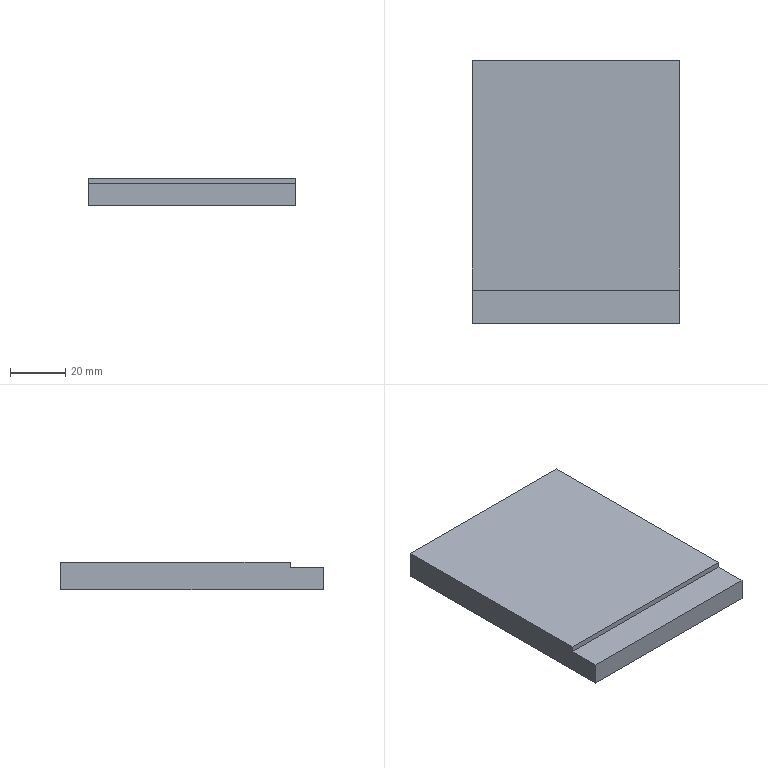Part | STEP file | 001-004-Feeding mechanism fixing plate | 1 solid | 8 faces | box 75 x 95 x 10 mm | volume 69450 mm3 | plane 8
STEP:
#1=CARTESIAN_POINT('',(0.,0.,0.));
#2=DIRECTION('',(0.,0.,1.));
#3=DIRECTION('',(1.,0.,0.));
#4=AXIS2_PLACEMENT_3D('',#1,#2,#3);
#5=CARTESIAN_POINT('',(37.5,-35.5,10.));
#6=VERTEX_POINT('',#5);
#7=CARTESIAN_POINT('',(37.5,47.5,10.));
#8=VERTEX_POINT('',#7);
#9=CARTESIAN_POINT('',(37.5,-47.5,10.));
#10=DIRECTION('',(0.,1.,0.));
#11=VECTOR('',#10,1.);
#12=LINE('',#9,#11);
#13=CARTESIAN_POINT('',(37.5,-47.5,10.));
#14=DIRECTION('',(-1.,0.,0.));
#15=DIRECTION('',(0.,0.,1.));
#16=AXIS2_PLACEMENT_3D('',#13,#14,#15);
#17=PLANE('',#16);
#18=CARTESIAN_POINT('',(0.,0.));
#19=DIRECTION('',(0.,1.));
#20=VECTOR('',#19,1.);
#21=LINE('',#18,#20);
#22=(GEOMETRIC_REPRESENTATION_CONTEXT(2)PARAMETRIC_REPRESENTATION_CONTEXT()REPRESENTATION_CONTEXT('',''));
#23=DEFINITIONAL_REPRESENTATION('',(#21),#22);
#24=PCURVE('',#17,#23);
#25=CARTESIAN_POINT('',(0.,0.,10.));
#26=DIRECTION('',(0.,0.,-1.));
#27=DIRECTION('',(-1.,0.,0.));
#28=AXIS2_PLACEMENT_3D('',#25,#26,#27);
#29=PLANE('',#28);
#30=CARTESIAN_POINT('',(-37.5,-47.5));
#31=DIRECTION('',(0.,1.));
#32=VECTOR('',#31,1.);
#33=LINE('',#30,#32);
#34=(GEOMETRIC_REPRESENTATION_CONTEXT(2)PARAMETRIC_REPRESENTATION_CONTEXT()REPRESENTATION_CONTEXT('',''));
#35=DEFINITIONAL_REPRESENTATION('',(#33),#34);
#36=PCURVE('',#29,#35);
#37=SURFACE_CURVE('',#12,(#24,#36),.PCURVE_S1.);
#38=EDGE_CURVE('',#6,#8,#37,.T.);
#39=ORIENTED_EDGE('',*,*,#38,.F.);
#40=CARTESIAN_POINT('',(37.5,-35.5,8.));
#41=VERTEX_POINT('',#40);
#42=CARTESIAN_POINT('',(37.5,-35.5,8.));
#43=DIRECTION('',(0.,0.,1.));
#44=VECTOR('',#43,1.);
#45=LINE('',#42,#44);
#46=CARTESIAN_POINT('',(-2.,12.));
#47=DIRECTION('',(1.,0.));
#48=VECTOR('',#47,1.);
#49=LINE('',#46,#48);
#50=(GEOMETRIC_REPRESENTATION_CONTEXT(2)PARAMETRIC_REPRESENTATION_CONTEXT()REPRESENTATION_CONTEXT('',''));
#51=DEFINITIONAL_REPRESENTATION('',(#49),#50);
#52=PCURVE('',#17,#51);
#53=CARTESIAN_POINT('',(-37.5,-35.5,8.));
#54=DIRECTION('',(0.,1.,0.));
#55=DIRECTION('',(0.,0.,1.));
#56=AXIS2_PLACEMENT_3D('',#53,#54,#55);
#57=PLANE('',#56);
#58=CARTESIAN_POINT('',(0.,75.));
#59=DIRECTION('',(1.,0.));
#60=VECTOR('',#59,1.);
#61=LINE('',#58,#60);
#62=(GEOMETRIC_REPRESENTATION_CONTEXT(2)PARAMETRIC_REPRESENTATION_CONTEXT()REPRESENTATION_CONTEXT('',''));
#63=DEFINITIONAL_REPRESENTATION('',(#61),#62);
#64=PCURVE('',#57,#63);
#65=SURFACE_CURVE('',#45,(#52,#64),.PCURVE_S1.);
#66=EDGE_CURVE('',#41,#6,#65,.T.);
#67=ORIENTED_EDGE('',*,*,#66,.F.);
#68=CARTESIAN_POINT('',(37.5,-47.5,8.));
#69=VERTEX_POINT('',#68);
#70=CARTESIAN_POINT('',(37.5,-47.5,8.));
#71=DIRECTION('',(0.,1.,0.));
#72=VECTOR('',#71,1.);
#73=LINE('',#70,#72);
#74=CARTESIAN_POINT('',(-2.,0.));
#75=DIRECTION('',(0.,1.));
#76=VECTOR('',#75,1.);
#77=LINE('',#74,#76);
#78=(GEOMETRIC_REPRESENTATION_CONTEXT(2)PARAMETRIC_REPRESENTATION_CONTEXT()REPRESENTATION_CONTEXT('',''));
#79=DEFINITIONAL_REPRESENTATION('',(#77),#78);
#80=PCURVE('',#17,#79);
#81=CARTESIAN_POINT('',(0.,0.,8.));
#82=DIRECTION('',(0.,0.,-1.));
#83=DIRECTION('',(-1.,0.,0.));
#84=AXIS2_PLACEMENT_3D('',#81,#82,#83);
#85=PLANE('',#84);
#86=CARTESIAN_POINT('',(-37.5,-47.5));
#87=DIRECTION('',(0.,1.));
#88=VECTOR('',#87,1.);
#89=LINE('',#86,#88);
#90=(GEOMETRIC_REPRESENTATION_CONTEXT(2)PARAMETRIC_REPRESENTATION_CONTEXT()REPRESENTATION_CONTEXT('',''));
#91=DEFINITIONAL_REPRESENTATION('',(#89),#90);
#92=PCURVE('',#85,#91);
#93=SURFACE_CURVE('',#73,(#80,#92),.PCURVE_S1.);
#94=EDGE_CURVE('',#69,#41,#93,.T.);
#95=ORIENTED_EDGE('',*,*,#94,.F.);
#96=CARTESIAN_POINT('',(37.5,-47.5,0.));
#97=VERTEX_POINT('',#96);
#98=CARTESIAN_POINT('',(37.5,-47.5,10.));
#99=DIRECTION('',(0.,0.,-1.));
#100=VECTOR('',#99,1.);
#101=LINE('',#98,#100);
#102=CARTESIAN_POINT('',(0.,0.));
#103=DIRECTION('',(-1.,0.));
#104=VECTOR('',#103,1.);
#105=LINE('',#102,#104);
#106=(GEOMETRIC_REPRESENTATION_CONTEXT(2)PARAMETRIC_REPRESENTATION_CONTEXT()REPRESENTATION_CONTEXT('',''));
#107=DEFINITIONAL_REPRESENTATION('',(#105),#106);
#108=PCURVE('',#17,#107);
#109=CARTESIAN_POINT('',(-37.5,-47.5,10.));
#110=DIRECTION('',(0.,1.,0.));
#111=DIRECTION('',(0.,0.,1.));
#112=AXIS2_PLACEMENT_3D('',#109,#110,#111);
#113=PLANE('',#112);
#114=CARTESIAN_POINT('',(0.,75.));
#115=DIRECTION('',(-1.,0.));
#116=VECTOR('',#115,1.);
#117=LINE('',#114,#116);
#118=(GEOMETRIC_REPRESENTATION_CONTEXT(2)PARAMETRIC_REPRESENTATION_CONTEXT()REPRESENTATION_CONTEXT('',''));
#119=DEFINITIONAL_REPRESENTATION('',(#117),#118);
#120=PCURVE('',#113,#119);
#121=SURFACE_CURVE('',#101,(#108,#120),.PCURVE_S1.);
#122=EDGE_CURVE('',#69,#97,#121,.T.);
#123=ORIENTED_EDGE('',*,*,#122,.T.);
#124=CARTESIAN_POINT('',(37.5,47.5,0.));
#125=VERTEX_POINT('',#124);
#126=CARTESIAN_POINT('',(37.5,-47.5,0.));
#127=DIRECTION('',(0.,1.,0.));
#128=VECTOR('',#127,1.);
#129=LINE('',#126,#128);
#130=CARTESIAN_POINT('',(-10.,0.));
#131=DIRECTION('',(0.,1.));
#132=VECTOR('',#131,1.);
#133=LINE('',#130,#132);
#134=(GEOMETRIC_REPRESENTATION_CONTEXT(2)PARAMETRIC_REPRESENTATION_CONTEXT()REPRESENTATION_CONTEXT('',''));
#135=DEFINITIONAL_REPRESENTATION('',(#133),#134);
#136=PCURVE('',#17,#135);
#137=CARTESIAN_POINT('',(0.,0.,0.));
#138=DIRECTION('',(0.,0.,-1.));
#139=DIRECTION('',(-1.,0.,0.));
#140=AXIS2_PLACEMENT_3D('',#137,#138,#139);
#141=PLANE('',#140);
#142=CARTESIAN_POINT('',(-37.5,-47.5));
#143=DIRECTION('',(0.,1.));
#144=VECTOR('',#143,1.);
#145=LINE('',#142,#144);
#146=(GEOMETRIC_REPRESENTATION_CONTEXT(2)PARAMETRIC_REPRESENTATION_CONTEXT()REPRESENTATION_CONTEXT('',''));
#147=DEFINITIONAL_REPRESENTATION('',(#145),#146);
#148=PCURVE('',#141,#147);
#149=SURFACE_CURVE('',#129,(#136,#148),.PCURVE_S1.);
#150=EDGE_CURVE('',#97,#125,#149,.T.);
#151=ORIENTED_EDGE('',*,*,#150,.T.);
#152=CARTESIAN_POINT('',(37.5,47.5,10.));
#153=DIRECTION('',(0.,0.,-1.));
#154=VECTOR('',#153,1.);
#155=LINE('',#152,#154);
#156=CARTESIAN_POINT('',(0.,95.));
#157=DIRECTION('',(-1.,0.));
#158=VECTOR('',#157,1.);
#159=LINE('',#156,#158);
#160=(GEOMETRIC_REPRESENTATION_CONTEXT(2)PARAMETRIC_REPRESENTATION_CONTEXT()REPRESENTATION_CONTEXT('',''));
#161=DEFINITIONAL_REPRESENTATION('',(#159),#160);
#162=PCURVE('',#17,#161);
#163=CARTESIAN_POINT('',(-37.5,47.5,10.));
#164=DIRECTION('',(0.,-1.,0.));
#165=DIRECTION('',(0.,0.,-1.));
#166=AXIS2_PLACEMENT_3D('',#163,#164,#165);
#167=PLANE('',#166);
#168=CARTESIAN_POINT('',(0.,75.));
#169=DIRECTION('',(1.,0.));
#170=VECTOR('',#169,1.);
#171=LINE('',#168,#170);
#172=(GEOMETRIC_REPRESENTATION_CONTEXT(2)PARAMETRIC_REPRESENTATION_CONTEXT()REPRESENTATION_CONTEXT('',''));
#173=DEFINITIONAL_REPRESENTATION('',(#171),#172);
#174=PCURVE('',#167,#173);
#175=SURFACE_CURVE('',#155,(#162,#174),.PCURVE_S1.);
#176=EDGE_CURVE('',#8,#125,#175,.T.);
#177=ORIENTED_EDGE('',*,*,#176,.F.);
#178=EDGE_LOOP('',(#39,#67,#95,#123,#151,#177));
#179=FACE_BOUND('',#178,.T.);
#180=ADVANCED_FACE('',(#179),#17,.F.);
#181=CARTESIAN_POINT('',(-37.5,47.5,0.));
#182=VERTEX_POINT('',#181);
#183=CARTESIAN_POINT('',(-37.5,47.5,0.));
#184=DIRECTION('',(-1.,0.,0.));
#185=VECTOR('',#184,1.);
#186=LINE('',#183,#185);
#187=CARTESIAN_POINT('',(10.,0.));
#188=DIRECTION('',(0.,-1.));
#189=VECTOR('',#188,1.);
#190=LINE('',#187,#189);
#191=(GEOMETRIC_REPRESENTATION_CONTEXT(2)PARAMETRIC_REPRESENTATION_CONTEXT()REPRESENTATION_CONTEXT('',''));
#192=DEFINITIONAL_REPRESENTATION('',(#190),#191);
#193=PCURVE('',#167,#192);
#194=CARTESIAN_POINT('',(37.5,47.5));
#195=DIRECTION('',(1.,0.));
#196=VECTOR('',#195,1.);
#197=LINE('',#194,#196);
#198=(GEOMETRIC_REPRESENTATION_CONTEXT(2)PARAMETRIC_REPRESENTATION_CONTEXT()REPRESENTATION_CONTEXT('',''));
#199=DEFINITIONAL_REPRESENTATION('',(#197),#198);
#200=PCURVE('',#141,#199);
#201=SURFACE_CURVE('',#186,(#193,#200),.PCURVE_S1.);
#202=EDGE_CURVE('',#125,#182,#201,.T.);
#203=ORIENTED_EDGE('',*,*,#202,.T.);
#204=CARTESIAN_POINT('',(-37.5,47.5,10.));
#205=VERTEX_POINT('',#204);
#206=CARTESIAN_POINT('',(-37.5,47.5,10.));
#207=DIRECTION('',(0.,0.,-1.));
#208=VECTOR('',#207,1.);
#209=LINE('',#206,#208);
#210=CARTESIAN_POINT('',(0.,0.));
#211=DIRECTION('',(1.,0.));
#212=VECTOR('',#211,1.);
#213=LINE('',#210,#212);
#214=(GEOMETRIC_REPRESENTATION_CONTEXT(2)PARAMETRIC_REPRESENTATION_CONTEXT()REPRESENTATION_CONTEXT('',''));
#215=DEFINITIONAL_REPRESENTATION('',(#213),#214);
#216=PCURVE('',#167,#215);
#217=CARTESIAN_POINT('',(-37.5,-47.5,10.));
#218=DIRECTION('',(1.,0.,0.));
#219=DIRECTION('',(0.,0.,-1.));
#220=AXIS2_PLACEMENT_3D('',#217,#218,#219);
#221=PLANE('',#220);
#222=CARTESIAN_POINT('',(0.,95.));
#223=DIRECTION('',(1.,0.));
#224=VECTOR('',#223,1.);
#225=LINE('',#222,#224);
#226=(GEOMETRIC_REPRESENTATION_CONTEXT(2)PARAMETRIC_REPRESENTATION_CONTEXT()REPRESENTATION_CONTEXT('',''));
#227=DEFINITIONAL_REPRESENTATION('',(#225),#226);
#228=PCURVE('',#221,#227);
#229=SURFACE_CURVE('',#209,(#216,#228),.PCURVE_S1.);
#230=EDGE_CURVE('',#205,#182,#229,.T.);
#231=ORIENTED_EDGE('',*,*,#230,.F.);
#232=CARTESIAN_POINT('',(-37.5,47.5,10.));
#233=DIRECTION('',(-1.,0.,0.));
#234=VECTOR('',#233,1.);
#235=LINE('',#232,#234);
#236=CARTESIAN_POINT('',(0.,0.));
#237=DIRECTION('',(0.,-1.));
#238=VECTOR('',#237,1.);
#239=LINE('',#236,#238);
#240=(GEOMETRIC_REPRESENTATION_CONTEXT(2)PARAMETRIC_REPRESENTATION_CONTEXT()REPRESENTATION_CONTEXT('',''));
#241=DEFINITIONAL_REPRESENTATION('',(#239),#240);
#242=PCURVE('',#167,#241);
#243=CARTESIAN_POINT('',(37.5,47.5));
#244=DIRECTION('',(1.,0.));
#245=VECTOR('',#244,1.);
#246=LINE('',#243,#245);
#247=(GEOMETRIC_REPRESENTATION_CONTEXT(2)PARAMETRIC_REPRESENTATION_CONTEXT()REPRESENTATION_CONTEXT('',''));
#248=DEFINITIONAL_REPRESENTATION('',(#246),#247);
#249=PCURVE('',#29,#248);
#250=SURFACE_CURVE('',#235,(#242,#249),.PCURVE_S1.);
#251=EDGE_CURVE('',#8,#205,#250,.T.);
#252=ORIENTED_EDGE('',*,*,#251,.F.);
#253=ORIENTED_EDGE('',*,*,#176,.T.);
#254=EDGE_LOOP('',(#203,#231,#252,#253));
#255=FACE_BOUND('',#254,.T.);
#256=ADVANCED_FACE('',(#255),#167,.F.);
#257=CARTESIAN_POINT('',(-37.5,-35.5,8.));
#258=VERTEX_POINT('',#257);
#259=CARTESIAN_POINT('',(-37.5,-47.5,8.));
#260=VERTEX_POINT('',#259);
#261=CARTESIAN_POINT('',(-37.5,-47.5,8.));
#262=DIRECTION('',(0.,-1.,0.));
#263=VECTOR('',#262,1.);
#264=LINE('',#261,#263);
#265=CARTESIAN_POINT('',(2.,0.));
#266=DIRECTION('',(0.,-1.));
#267=VECTOR('',#266,1.);
#268=LINE('',#265,#267);
#269=(GEOMETRIC_REPRESENTATION_CONTEXT(2)PARAMETRIC_REPRESENTATION_CONTEXT()REPRESENTATION_CONTEXT('',''));
#270=DEFINITIONAL_REPRESENTATION('',(#268),#269);
#271=PCURVE('',#221,#270);
#272=CARTESIAN_POINT('',(37.5,-47.5));
#273=DIRECTION('',(0.,-1.));
#274=VECTOR('',#273,1.);
#275=LINE('',#272,#274);
#276=(GEOMETRIC_REPRESENTATION_CONTEXT(2)PARAMETRIC_REPRESENTATION_CONTEXT()REPRESENTATION_CONTEXT('',''));
#277=DEFINITIONAL_REPRESENTATION('',(#275),#276);
#278=PCURVE('',#85,#277);
#279=SURFACE_CURVE('',#264,(#271,#278),.PCURVE_S1.);
#280=EDGE_CURVE('',#258,#260,#279,.T.);
#281=ORIENTED_EDGE('',*,*,#280,.F.);
#282=CARTESIAN_POINT('',(-37.5,-35.5,10.));
#283=VERTEX_POINT('',#282);
#284=CARTESIAN_POINT('',(-37.5,-35.5,8.));
#285=DIRECTION('',(0.,0.,1.));
#286=VECTOR('',#285,1.);
#287=LINE('',#284,#286);
#288=CARTESIAN_POINT('',(2.,12.));
#289=DIRECTION('',(-1.,0.));
#290=VECTOR('',#289,1.);
#291=LINE('',#288,#290);
#292=(GEOMETRIC_REPRESENTATION_CONTEXT(2)PARAMETRIC_REPRESENTATION_CONTEXT()REPRESENTATION_CONTEXT('',''));
#293=DEFINITIONAL_REPRESENTATION('',(#291),#292);
#294=PCURVE('',#221,#293);
#295=CARTESIAN_POINT('',(0.,0.));
#296=DIRECTION('',(1.,0.));
#297=VECTOR('',#296,1.);
#298=LINE('',#295,#297);
#299=(GEOMETRIC_REPRESENTATION_CONTEXT(2)PARAMETRIC_REPRESENTATION_CONTEXT()REPRESENTATION_CONTEXT('',''));
#300=DEFINITIONAL_REPRESENTATION('',(#298),#299);
#301=PCURVE('',#57,#300);
#302=SURFACE_CURVE('',#287,(#294,#301),.PCURVE_S1.);
#303=EDGE_CURVE('',#258,#283,#302,.T.);
#304=ORIENTED_EDGE('',*,*,#303,.T.);
#305=CARTESIAN_POINT('',(-37.5,-47.5,10.));
#306=DIRECTION('',(0.,-1.,0.));
#307=VECTOR('',#306,1.);
#308=LINE('',#305,#307);
#309=CARTESIAN_POINT('',(0.,0.));
#310=DIRECTION('',(0.,-1.));
#311=VECTOR('',#310,1.);
#312=LINE('',#309,#311);
#313=(GEOMETRIC_REPRESENTATION_CONTEXT(2)PARAMETRIC_REPRESENTATION_CONTEXT()REPRESENTATION_CONTEXT('',''));
#314=DEFINITIONAL_REPRESENTATION('',(#312),#313);
#315=PCURVE('',#221,#314);
#316=CARTESIAN_POINT('',(37.5,-47.5));
#317=DIRECTION('',(0.,-1.));
#318=VECTOR('',#317,1.);
#319=LINE('',#316,#318);
#320=(GEOMETRIC_REPRESENTATION_CONTEXT(2)PARAMETRIC_REPRESENTATION_CONTEXT()REPRESENTATION_CONTEXT('',''));
#321=DEFINITIONAL_REPRESENTATION('',(#319),#320);
#322=PCURVE('',#29,#321);
#323=SURFACE_CURVE('',#308,(#315,#322),.PCURVE_S1.);
#324=EDGE_CURVE('',#205,#283,#323,.T.);
#325=ORIENTED_EDGE('',*,*,#324,.F.);
#326=ORIENTED_EDGE('',*,*,#230,.T.);
#327=CARTESIAN_POINT('',(-37.5,-47.5,0.));
#328=VERTEX_POINT('',#327);
#329=CARTESIAN_POINT('',(-37.5,-47.5,0.));
#330=DIRECTION('',(0.,-1.,0.));
#331=VECTOR('',#330,1.);
#332=LINE('',#329,#331);
#333=CARTESIAN_POINT('',(10.,0.));
#334=DIRECTION('',(0.,-1.));
#335=VECTOR('',#334,1.);
#336=LINE('',#333,#335);
#337=(GEOMETRIC_REPRESENTATION_CONTEXT(2)PARAMETRIC_REPRESENTATION_CONTEXT()REPRESENTATION_CONTEXT('',''));
#338=DEFINITIONAL_REPRESENTATION('',(#336),#337);
#339=PCURVE('',#221,#338);
#340=CARTESIAN_POINT('',(37.5,-47.5));
#341=DIRECTION('',(0.,-1.));
#342=VECTOR('',#341,1.);
#343=LINE('',#340,#342);
#344=(GEOMETRIC_REPRESENTATION_CONTEXT(2)PARAMETRIC_REPRESENTATION_CONTEXT()REPRESENTATION_CONTEXT('',''));
#345=DEFINITIONAL_REPRESENTATION('',(#343),#344);
#346=PCURVE('',#141,#345);
#347=SURFACE_CURVE('',#332,(#339,#346),.PCURVE_S1.);
#348=EDGE_CURVE('',#182,#328,#347,.T.);
#349=ORIENTED_EDGE('',*,*,#348,.T.);
#350=CARTESIAN_POINT('',(-37.5,-47.5,10.));
#351=DIRECTION('',(0.,0.,-1.));
#352=VECTOR('',#351,1.);
#353=LINE('',#350,#352);
#354=CARTESIAN_POINT('',(0.,0.));
#355=DIRECTION('',(1.,0.));
#356=VECTOR('',#355,1.);
#357=LINE('',#354,#356);
#358=(GEOMETRIC_REPRESENTATION_CONTEXT(2)PARAMETRIC_REPRESENTATION_CONTEXT()REPRESENTATION_CONTEXT('',''));
#359=DEFINITIONAL_REPRESENTATION('',(#357),#358);
#360=PCURVE('',#221,#359);
#361=CARTESIAN_POINT('',(0.,0.));
#362=DIRECTION('',(-1.,0.));
#363=VECTOR('',#362,1.);
#364=LINE('',#361,#363);
#365=(GEOMETRIC_REPRESENTATION_CONTEXT(2)PARAMETRIC_REPRESENTATION_CONTEXT()REPRESENTATION_CONTEXT('',''));
#366=DEFINITIONAL_REPRESENTATION('',(#364),#365);
#367=PCURVE('',#113,#366);
#368=SURFACE_CURVE('',#353,(#360,#367),.PCURVE_S1.);
#369=EDGE_CURVE('',#260,#328,#368,.T.);
#370=ORIENTED_EDGE('',*,*,#369,.F.);
#371=EDGE_LOOP('',(#281,#304,#325,#326,#349,#370));
#372=FACE_BOUND('',#371,.T.);
#373=ADVANCED_FACE('',(#372),#221,.F.);
#374=ORIENTED_EDGE('',*,*,#122,.F.);
#375=CARTESIAN_POINT('',(-37.5,-47.5,8.));
#376=DIRECTION('',(1.,0.,0.));
#377=VECTOR('',#376,1.);
#378=LINE('',#375,#377);
#379=CARTESIAN_POINT('',(-2.,0.));
#380=DIRECTION('',(0.,1.));
#381=VECTOR('',#380,1.);
#382=LINE('',#379,#381);
#383=(GEOMETRIC_REPRESENTATION_CONTEXT(2)PARAMETRIC_REPRESENTATION_CONTEXT()REPRESENTATION_CONTEXT('',''));
#384=DEFINITIONAL_REPRESENTATION('',(#382),#383);
#385=PCURVE('',#113,#384);
#386=CARTESIAN_POINT('',(37.5,-47.5));
#387=DIRECTION('',(-1.,0.));
#388=VECTOR('',#387,1.);
#389=LINE('',#386,#388);
#390=(GEOMETRIC_REPRESENTATION_CONTEXT(2)PARAMETRIC_REPRESENTATION_CONTEXT()REPRESENTATION_CONTEXT('',''));
#391=DEFINITIONAL_REPRESENTATION('',(#389),#390);
#392=PCURVE('',#85,#391);
#393=SURFACE_CURVE('',#378,(#385,#392),.PCURVE_S1.);
#394=EDGE_CURVE('',#260,#69,#393,.T.);
#395=ORIENTED_EDGE('',*,*,#394,.F.);
#396=ORIENTED_EDGE('',*,*,#369,.T.);
#397=CARTESIAN_POINT('',(-37.5,-47.5,0.));
#398=DIRECTION('',(1.,0.,0.));
#399=VECTOR('',#398,1.);
#400=LINE('',#397,#399);
#401=CARTESIAN_POINT('',(-10.,0.));
#402=DIRECTION('',(0.,1.));
#403=VECTOR('',#402,1.);
#404=LINE('',#401,#403);
#405=(GEOMETRIC_REPRESENTATION_CONTEXT(2)PARAMETRIC_REPRESENTATION_CONTEXT()REPRESENTATION_CONTEXT('',''));
#406=DEFINITIONAL_REPRESENTATION('',(#404),#405);
#407=PCURVE('',#113,#406);
#408=CARTESIAN_POINT('',(37.5,-47.5));
#409=DIRECTION('',(-1.,0.));
#410=VECTOR('',#409,1.);
#411=LINE('',#408,#410);
#412=(GEOMETRIC_REPRESENTATION_CONTEXT(2)PARAMETRIC_REPRESENTATION_CONTEXT()REPRESENTATION_CONTEXT('',''));
#413=DEFINITIONAL_REPRESENTATION('',(#411),#412);
#414=PCURVE('',#141,#413);
#415=SURFACE_CURVE('',#400,(#407,#414),.PCURVE_S1.);
#416=EDGE_CURVE('',#328,#97,#415,.T.);
#417=ORIENTED_EDGE('',*,*,#416,.T.);
#418=EDGE_LOOP('',(#374,#395,#396,#417));
#419=FACE_BOUND('',#418,.T.);
#420=ADVANCED_FACE('',(#419),#113,.F.);
#421=ORIENTED_EDGE('',*,*,#324,.T.);
#422=CARTESIAN_POINT('',(-37.5,-35.5,10.));
#423=DIRECTION('',(-1.,0.,0.));
#424=VECTOR('',#423,1.);
#425=LINE('',#422,#424);
#426=CARTESIAN_POINT('',(37.5,-35.5));
#427=DIRECTION('',(1.,0.));
#428=VECTOR('',#427,1.);
#429=LINE('',#426,#428);
#430=(GEOMETRIC_REPRESENTATION_CONTEXT(2)PARAMETRIC_REPRESENTATION_CONTEXT()REPRESENTATION_CONTEXT('',''));
#431=DEFINITIONAL_REPRESENTATION('',(#429),#430);
#432=PCURVE('',#29,#431);
#433=CARTESIAN_POINT('',(2.,0.));
#434=DIRECTION('',(0.,-1.));
#435=VECTOR('',#434,1.);
#436=LINE('',#433,#435);
#437=(GEOMETRIC_REPRESENTATION_CONTEXT(2)PARAMETRIC_REPRESENTATION_CONTEXT()REPRESENTATION_CONTEXT('',''));
#438=DEFINITIONAL_REPRESENTATION('',(#436),#437);
#439=PCURVE('',#57,#438);
#440=SURFACE_CURVE('',#425,(#432,#439),.PCURVE_S1.);
#441=EDGE_CURVE('',#6,#283,#440,.T.);
#442=ORIENTED_EDGE('',*,*,#441,.F.);
#443=ORIENTED_EDGE('',*,*,#38,.T.);
#444=ORIENTED_EDGE('',*,*,#251,.T.);
#445=EDGE_LOOP('',(#421,#442,#443,#444));
#446=FACE_BOUND('',#445,.T.);
#447=ADVANCED_FACE('',(#446),#29,.F.);
#448=ORIENTED_EDGE('',*,*,#150,.F.);
#449=ORIENTED_EDGE('',*,*,#416,.F.);
#450=ORIENTED_EDGE('',*,*,#348,.F.);
#451=ORIENTED_EDGE('',*,*,#202,.F.);
#452=EDGE_LOOP('',(#448,#449,#450,#451));
#453=FACE_BOUND('',#452,.T.);
#454=ADVANCED_FACE('',(#453),#141,.T.);
#455=ORIENTED_EDGE('',*,*,#441,.T.);
#456=ORIENTED_EDGE('',*,*,#303,.F.);
#457=CARTESIAN_POINT('',(-37.5,-35.5,8.));
#458=DIRECTION('',(-1.,0.,0.));
#459=VECTOR('',#458,1.);
#460=LINE('',#457,#459);
#461=CARTESIAN_POINT('',(0.,0.));
#462=DIRECTION('',(0.,-1.));
#463=VECTOR('',#462,1.);
#464=LINE('',#461,#463);
#465=(GEOMETRIC_REPRESENTATION_CONTEXT(2)PARAMETRIC_REPRESENTATION_CONTEXT()REPRESENTATION_CONTEXT('',''));
#466=DEFINITIONAL_REPRESENTATION('',(#464),#465);
#467=PCURVE('',#57,#466);
#468=CARTESIAN_POINT('',(37.5,-35.5));
#469=DIRECTION('',(1.,0.));
#470=VECTOR('',#469,1.);
#471=LINE('',#468,#470);
#472=(GEOMETRIC_REPRESENTATION_CONTEXT(2)PARAMETRIC_REPRESENTATION_CONTEXT()REPRESENTATION_CONTEXT('',''));
#473=DEFINITIONAL_REPRESENTATION('',(#471),#472);
#474=PCURVE('',#85,#473);
#475=SURFACE_CURVE('',#460,(#467,#474),.PCURVE_S1.);
#476=EDGE_CURVE('',#41,#258,#475,.T.);
#477=ORIENTED_EDGE('',*,*,#476,.F.);
#478=ORIENTED_EDGE('',*,*,#66,.T.);
#479=EDGE_LOOP('',(#455,#456,#477,#478));
#480=FACE_BOUND('',#479,.T.);
#481=ADVANCED_FACE('',(#480),#57,.F.);
#482=ORIENTED_EDGE('',*,*,#280,.T.);
#483=ORIENTED_EDGE('',*,*,#394,.T.);
#484=ORIENTED_EDGE('',*,*,#94,.T.);
#485=ORIENTED_EDGE('',*,*,#476,.T.);
#486=EDGE_LOOP('',(#482,#483,#484,#485));
#487=FACE_BOUND('',#486,.T.);
#488=ADVANCED_FACE('',(#487),#85,.F.);
#489=CLOSED_SHELL('',(#180,#256,#373,#420,#447,#454,#481,#488));
#490=MANIFOLD_SOLID_BREP('',#489);
#491=(LENGTH_UNIT()NAMED_UNIT(*)SI_UNIT(.MILLI.,.METRE.));
#492=UNCERTAINTY_MEASURE_WITH_UNIT(LENGTH_MEASURE(0.0000001),#491,'','');
#493=(NAMED_UNIT(*)PLANE_ANGLE_UNIT()SI_UNIT($,.RADIAN.));
#494=(NAMED_UNIT(*)SI_UNIT($,.STERADIAN.)SOLID_ANGLE_UNIT());
#495=(GEOMETRIC_REPRESENTATION_CONTEXT(3)GLOBAL_UNCERTAINTY_ASSIGNED_CONTEXT((#492))GLOBAL_UNIT_ASSIGNED_CONTEXT((#491,#493,#494))REPRESENTATION_CONTEXT('',''));
#496=ADVANCED_BREP_SHAPE_REPRESENTATION('',(#4,#490),#495);